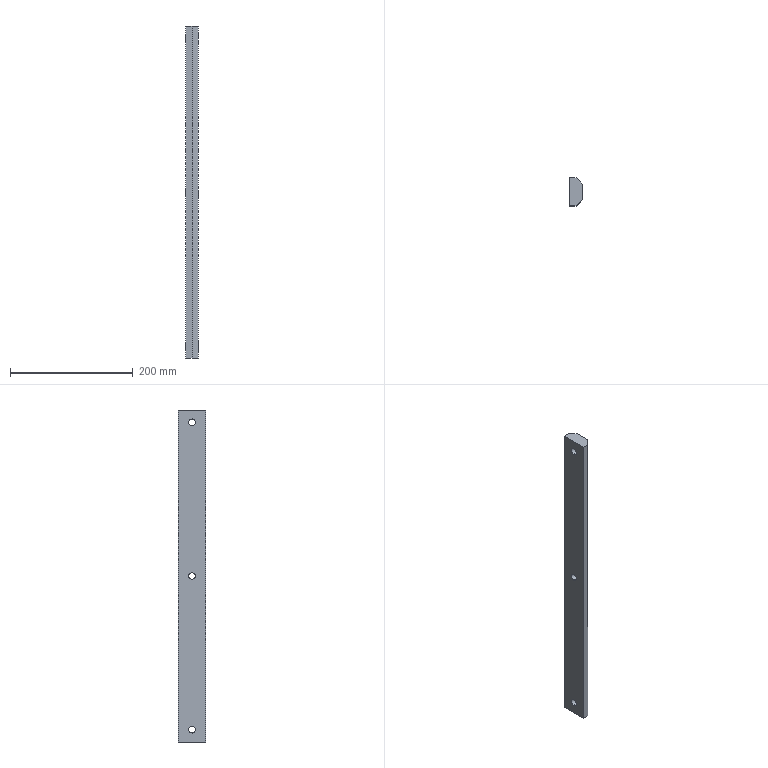Part | STEP file | PN_0008 | 1 solid | 23 faces | box 20 x 45 x 540 mm | volume 420510 mm3 | cylinder 12 | plane 11 | commonest cylinder face diameters 11 x6 18 x6